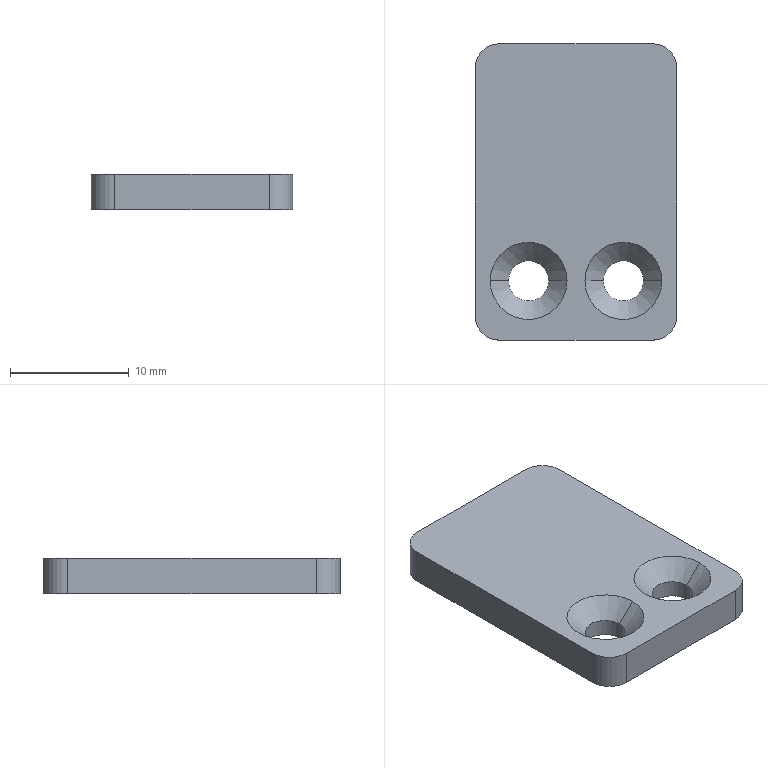Part | NX | features BREP 1 | 1 solid | 18 faces | box 17 x 25 x 3 mm | volume 1177 mm3 | cylinder 8 | plane 6 | cone 4 | commonest cylinder face diameters 3.4 x4 4 x4
STEP:
#1=CARTESIAN_POINT('',(-8.5,10.5,-3.));
#2=VERTEX_POINT('',#1);
#3=CARTESIAN_POINT('',(-6.5,12.5,-3.));
#4=VERTEX_POINT('',#3);
#5=CARTESIAN_POINT('',(-6.5,10.5,-3.));
#6=DIRECTION('',(0.,0.,-1.));
#7=DIRECTION('',(-1.,0.,0.));
#8=AXIS2_PLACEMENT_3D('',#5,#6,#7);
#9=CIRCLE('',#8,2.);
#10=EDGE_CURVE('',#2,#4,#9,.T.);
#11=ORIENTED_EDGE('',*,*,#10,.F.);
#12=CARTESIAN_POINT('',(-8.5,10.5,0.));
#13=VERTEX_POINT('',#12);
#14=CARTESIAN_POINT('',(-8.5,10.5,-3.));
#15=DIRECTION('',(0.,0.,-1.));
#16=VECTOR('',#15,1000.);
#17=LINE('',#14,#16);
#18=EDGE_CURVE('',#13,#2,#17,.T.);
#19=ORIENTED_EDGE('',*,*,#18,.F.);
#20=CARTESIAN_POINT('',(-6.5,12.5,0.));
#21=VERTEX_POINT('',#20);
#22=CARTESIAN_POINT('',(-6.5,10.5,0.));
#23=DIRECTION('',(0.,0.,1.));
#24=DIRECTION('',(-1.,0.,0.));
#25=AXIS2_PLACEMENT_3D('',#22,#23,#24);
#26=CIRCLE('',#25,2.);
#27=EDGE_CURVE('',#21,#13,#26,.T.);
#28=ORIENTED_EDGE('',*,*,#27,.F.);
#29=CARTESIAN_POINT('',(-6.5,12.5,-3.));
#30=DIRECTION('',(0.,0.,1.));
#31=VECTOR('',#30,1000.);
#32=LINE('',#29,#31);
#33=EDGE_CURVE('',#4,#21,#32,.T.);
#34=ORIENTED_EDGE('',*,*,#33,.F.);
#35=EDGE_LOOP('',(#11,#19,#28,#34));
#36=FACE_BOUND('',#35,.T.);
#37=CARTESIAN_POINT('',(-6.5,10.5,-3.));
#38=DIRECTION('',(0.,0.,1.));
#39=DIRECTION('',(1.,0.,0.));
#40=AXIS2_PLACEMENT_3D('',#37,#38,#39);
#41=CYLINDRICAL_SURFACE('',#40,2.);
#42=ADVANCED_FACE('',(#36),#41,.T.);
#43=CARTESIAN_POINT('',(6.5,12.5,-3.));
#44=VERTEX_POINT('',#43);
#45=CARTESIAN_POINT('',(8.5,10.5,-3.));
#46=VERTEX_POINT('',#45);
#47=CARTESIAN_POINT('',(6.5,10.5,-3.));
#48=DIRECTION('',(0.,0.,-1.));
#49=DIRECTION('',(-1.,0.,0.));
#50=AXIS2_PLACEMENT_3D('',#47,#48,#49);
#51=CIRCLE('',#50,2.);
#52=EDGE_CURVE('',#44,#46,#51,.T.);
#53=ORIENTED_EDGE('',*,*,#52,.F.);
#54=CARTESIAN_POINT('',(6.5,12.5,0.));
#55=VERTEX_POINT('',#54);
#56=CARTESIAN_POINT('',(6.5,12.5,-3.));
#57=DIRECTION('',(0.,0.,-1.));
#58=VECTOR('',#57,1000.);
#59=LINE('',#56,#58);
#60=EDGE_CURVE('',#55,#44,#59,.T.);
#61=ORIENTED_EDGE('',*,*,#60,.F.);
#62=CARTESIAN_POINT('',(8.5,10.5,0.));
#63=VERTEX_POINT('',#62);
#64=CARTESIAN_POINT('',(6.5,10.5,0.));
#65=DIRECTION('',(0.,0.,1.));
#66=DIRECTION('',(-1.,0.,0.));
#67=AXIS2_PLACEMENT_3D('',#64,#65,#66);
#68=CIRCLE('',#67,2.);
#69=EDGE_CURVE('',#63,#55,#68,.T.);
#70=ORIENTED_EDGE('',*,*,#69,.F.);
#71=CARTESIAN_POINT('',(8.5,10.5,-3.));
#72=DIRECTION('',(0.,0.,1.));
#73=VECTOR('',#72,1000.);
#74=LINE('',#71,#73);
#75=EDGE_CURVE('',#46,#63,#74,.T.);
#76=ORIENTED_EDGE('',*,*,#75,.F.);
#77=EDGE_LOOP('',(#53,#61,#70,#76));
#78=FACE_BOUND('',#77,.T.);
#79=CARTESIAN_POINT('',(6.5,10.5,-3.));
#80=DIRECTION('',(0.,0.,1.));
#81=DIRECTION('',(1.,0.,0.));
#82=AXIS2_PLACEMENT_3D('',#79,#80,#81);
#83=CYLINDRICAL_SURFACE('',#82,2.);
#84=ADVANCED_FACE('',(#78),#83,.T.);
#85=CARTESIAN_POINT('',(-6.5,-12.5,-3.));
#86=VERTEX_POINT('',#85);
#87=CARTESIAN_POINT('',(-8.5,-10.5,-3.));
#88=VERTEX_POINT('',#87);
#89=CARTESIAN_POINT('',(-6.5,-10.5,-3.));
#90=DIRECTION('',(0.,0.,-1.));
#91=DIRECTION('',(-1.,0.,0.));
#92=AXIS2_PLACEMENT_3D('',#89,#90,#91);
#93=CIRCLE('',#92,2.);
#94=EDGE_CURVE('',#86,#88,#93,.T.);
#95=ORIENTED_EDGE('',*,*,#94,.F.);
#96=CARTESIAN_POINT('',(-6.5,-12.5,0.));
#97=VERTEX_POINT('',#96);
#98=CARTESIAN_POINT('',(-6.5,-12.5,-3.));
#99=DIRECTION('',(0.,0.,-1.));
#100=VECTOR('',#99,1000.);
#101=LINE('',#98,#100);
#102=EDGE_CURVE('',#97,#86,#101,.T.);
#103=ORIENTED_EDGE('',*,*,#102,.F.);
#104=CARTESIAN_POINT('',(-8.5,-10.5,0.));
#105=VERTEX_POINT('',#104);
#106=CARTESIAN_POINT('',(-6.5,-10.5,0.));
#107=DIRECTION('',(0.,0.,1.));
#108=DIRECTION('',(-1.,0.,0.));
#109=AXIS2_PLACEMENT_3D('',#106,#107,#108);
#110=CIRCLE('',#109,2.);
#111=EDGE_CURVE('',#105,#97,#110,.T.);
#112=ORIENTED_EDGE('',*,*,#111,.F.);
#113=CARTESIAN_POINT('',(-8.5,-10.5,-3.));
#114=DIRECTION('',(0.,0.,1.));
#115=VECTOR('',#114,1000.);
#116=LINE('',#113,#115);
#117=EDGE_CURVE('',#88,#105,#116,.T.);
#118=ORIENTED_EDGE('',*,*,#117,.F.);
#119=EDGE_LOOP('',(#95,#103,#112,#118));
#120=FACE_BOUND('',#119,.T.);
#121=CARTESIAN_POINT('',(-6.5,-10.5,-3.));
#122=DIRECTION('',(0.,0.,1.));
#123=DIRECTION('',(1.,0.,0.));
#124=AXIS2_PLACEMENT_3D('',#121,#122,#123);
#125=CYLINDRICAL_SURFACE('',#124,2.);
#126=ADVANCED_FACE('',(#120),#125,.T.);
#127=CARTESIAN_POINT('',(8.5,-10.5,-3.));
#128=VERTEX_POINT('',#127);
#129=CARTESIAN_POINT('',(6.5,-12.5,-3.));
#130=VERTEX_POINT('',#129);
#131=CARTESIAN_POINT('',(6.5,-10.5,-3.));
#132=DIRECTION('',(0.,0.,-1.));
#133=DIRECTION('',(-1.,0.,0.));
#134=AXIS2_PLACEMENT_3D('',#131,#132,#133);
#135=CIRCLE('',#134,2.);
#136=EDGE_CURVE('',#128,#130,#135,.T.);
#137=ORIENTED_EDGE('',*,*,#136,.F.);
#138=CARTESIAN_POINT('',(8.5,-10.5,0.));
#139=VERTEX_POINT('',#138);
#140=CARTESIAN_POINT('',(8.5,-10.5,-3.));
#141=DIRECTION('',(0.,0.,-1.));
#142=VECTOR('',#141,1000.);
#143=LINE('',#140,#142);
#144=EDGE_CURVE('',#139,#128,#143,.T.);
#145=ORIENTED_EDGE('',*,*,#144,.F.);
#146=CARTESIAN_POINT('',(6.5,-12.5,0.));
#147=VERTEX_POINT('',#146);
#148=CARTESIAN_POINT('',(6.5,-10.5,0.));
#149=DIRECTION('',(0.,0.,1.));
#150=DIRECTION('',(-1.,0.,0.));
#151=AXIS2_PLACEMENT_3D('',#148,#149,#150);
#152=CIRCLE('',#151,2.);
#153=EDGE_CURVE('',#147,#139,#152,.T.);
#154=ORIENTED_EDGE('',*,*,#153,.F.);
#155=CARTESIAN_POINT('',(6.5,-12.5,-3.));
#156=DIRECTION('',(0.,0.,1.));
#157=VECTOR('',#156,1000.);
#158=LINE('',#155,#157);
#159=EDGE_CURVE('',#130,#147,#158,.T.);
#160=ORIENTED_EDGE('',*,*,#159,.F.);
#161=EDGE_LOOP('',(#137,#145,#154,#160));
#162=FACE_BOUND('',#161,.T.);
#163=CARTESIAN_POINT('',(6.5,-10.5,-3.));
#164=DIRECTION('',(0.,0.,1.));
#165=DIRECTION('',(1.,0.,0.));
#166=AXIS2_PLACEMENT_3D('',#163,#164,#165);
#167=CYLINDRICAL_SURFACE('',#166,2.);
#168=ADVANCED_FACE('',(#162),#167,.T.);
#169=CARTESIAN_POINT('',(-7.25,-7.5,0.));
#170=VERTEX_POINT('',#169);
#171=CARTESIAN_POINT('',(-5.7,-7.5,-1.55));
#172=VERTEX_POINT('',#171);
#173=CARTESIAN_POINT('',(-7.25,-7.5,0.));
#174=DIRECTION('',(-0.7071,0.,0.7071));
#175=VECTOR('',#174,1000.);
#176=LINE('',#173,#175);
#177=EDGE_CURVE('',#170,#172,#176,.F.);
#178=ORIENTED_EDGE('',*,*,#177,.T.);
#179=CARTESIAN_POINT('',(-2.3,-7.5,-1.55));
#180=VERTEX_POINT('',#179);
#181=CARTESIAN_POINT('',(-4.,-7.5,-1.55));
#182=DIRECTION('',(0.,0.,1.));
#183=DIRECTION('',(1.,0.,0.));
#184=AXIS2_PLACEMENT_3D('',#181,#182,#183);
#185=CIRCLE('',#184,1.7);
#186=EDGE_CURVE('',#180,#172,#185,.T.);
#187=ORIENTED_EDGE('',*,*,#186,.F.);
#188=CARTESIAN_POINT('',(-0.75,-7.5,0.));
#189=VERTEX_POINT('',#188);
#190=CARTESIAN_POINT('',(-0.75,-7.5,0.));
#191=DIRECTION('',(0.7071,0.,0.7071));
#192=VECTOR('',#191,1000.);
#193=LINE('',#190,#192);
#194=EDGE_CURVE('',#189,#180,#193,.F.);
#195=ORIENTED_EDGE('',*,*,#194,.F.);
#196=CARTESIAN_POINT('',(-4.,-7.5,0.));
#197=DIRECTION('',(0.,0.,1.));
#198=DIRECTION('',(1.,0.,0.));
#199=AXIS2_PLACEMENT_3D('',#196,#197,#198);
#200=CIRCLE('',#199,3.25);
#201=EDGE_CURVE('',#189,#170,#200,.T.);
#202=ORIENTED_EDGE('',*,*,#201,.T.);
#203=EDGE_LOOP('',(#178,#187,#195,#202));
#204=FACE_BOUND('',#203,.T.);
#205=CARTESIAN_POINT('',(-4.,-7.5,0.));
#206=DIRECTION('',(0.,0.,1.));
#207=DIRECTION('',(1.,0.,0.));
#208=AXIS2_PLACEMENT_3D('',#205,#206,#207);
#209=CONICAL_SURFACE('',#208,3.25,0.7854);
#210=ADVANCED_FACE('',(#204),#209,.F.);
#211=CARTESIAN_POINT('',(-5.7,-7.5,-3.));
#212=VERTEX_POINT('',#211);
#213=CARTESIAN_POINT('',(-5.7,-7.5,0.));
#214=DIRECTION('',(0.,0.,1.));
#215=VECTOR('',#214,1000.);
#216=LINE('',#213,#215);
#217=EDGE_CURVE('',#172,#212,#216,.F.);
#218=ORIENTED_EDGE('',*,*,#217,.T.);
#219=CARTESIAN_POINT('',(-2.3,-7.5,-3.));
#220=VERTEX_POINT('',#219);
#221=CARTESIAN_POINT('',(-4.,-7.5,-3.));
#222=DIRECTION('',(0.,0.,-1.));
#223=DIRECTION('',(-1.,0.,0.));
#224=AXIS2_PLACEMENT_3D('',#221,#222,#223);
#225=CIRCLE('',#224,1.7);
#226=EDGE_CURVE('',#212,#220,#225,.T.);
#227=ORIENTED_EDGE('',*,*,#226,.T.);
#228=CARTESIAN_POINT('',(-2.3,-7.5,0.));
#229=DIRECTION('',(0.,0.,1.));
#230=VECTOR('',#229,1000.);
#231=LINE('',#228,#230);
#232=EDGE_CURVE('',#180,#220,#231,.F.);
#233=ORIENTED_EDGE('',*,*,#232,.F.);
#234=ORIENTED_EDGE('',*,*,#186,.T.);
#235=EDGE_LOOP('',(#218,#227,#233,#234));
#236=FACE_BOUND('',#235,.T.);
#237=CARTESIAN_POINT('',(-4.,-7.5,0.));
#238=DIRECTION('',(0.,0.,1.));
#239=DIRECTION('',(1.,0.,0.));
#240=AXIS2_PLACEMENT_3D('',#237,#238,#239);
#241=CYLINDRICAL_SURFACE('',#240,1.7);
#242=ADVANCED_FACE('',(#236),#241,.F.);
#243=CARTESIAN_POINT('',(0.75,-7.5,0.));
#244=VERTEX_POINT('',#243);
#245=CARTESIAN_POINT('',(2.3,-7.5,-1.55));
#246=VERTEX_POINT('',#245);
#247=CARTESIAN_POINT('',(0.75,-7.5,0.));
#248=DIRECTION('',(-0.7071,0.,0.7071));
#249=VECTOR('',#248,1000.);
#250=LINE('',#247,#249);
#251=EDGE_CURVE('',#244,#246,#250,.F.);
#252=ORIENTED_EDGE('',*,*,#251,.T.);
#253=CARTESIAN_POINT('',(5.7,-7.5,-1.55));
#254=VERTEX_POINT('',#253);
#255=CARTESIAN_POINT('',(4.,-7.5,-1.55));
#256=DIRECTION('',(0.,0.,1.));
#257=DIRECTION('',(1.,0.,0.));
#258=AXIS2_PLACEMENT_3D('',#255,#256,#257);
#259=CIRCLE('',#258,1.7);
#260=EDGE_CURVE('',#254,#246,#259,.T.);
#261=ORIENTED_EDGE('',*,*,#260,.F.);
#262=CARTESIAN_POINT('',(7.25,-7.5,0.));
#263=VERTEX_POINT('',#262);
#264=CARTESIAN_POINT('',(7.25,-7.5,0.));
#265=DIRECTION('',(0.7071,0.,0.7071));
#266=VECTOR('',#265,1000.);
#267=LINE('',#264,#266);
#268=EDGE_CURVE('',#263,#254,#267,.F.);
#269=ORIENTED_EDGE('',*,*,#268,.F.);
#270=CARTESIAN_POINT('',(4.,-7.5,0.));
#271=DIRECTION('',(0.,0.,1.));
#272=DIRECTION('',(1.,0.,0.));
#273=AXIS2_PLACEMENT_3D('',#270,#271,#272);
#274=CIRCLE('',#273,3.25);
#275=EDGE_CURVE('',#263,#244,#274,.T.);
#276=ORIENTED_EDGE('',*,*,#275,.T.);
#277=EDGE_LOOP('',(#252,#261,#269,#276));
#278=FACE_BOUND('',#277,.T.);
#279=CARTESIAN_POINT('',(4.,-7.5,0.));
#280=DIRECTION('',(0.,0.,1.));
#281=DIRECTION('',(1.,0.,0.));
#282=AXIS2_PLACEMENT_3D('',#279,#280,#281);
#283=CONICAL_SURFACE('',#282,3.25,0.7854);
#284=ADVANCED_FACE('',(#278),#283,.F.);
#285=CARTESIAN_POINT('',(2.3,-7.5,-3.));
#286=VERTEX_POINT('',#285);
#287=CARTESIAN_POINT('',(2.3,-7.5,0.));
#288=DIRECTION('',(0.,0.,1.));
#289=VECTOR('',#288,1000.);
#290=LINE('',#287,#289);
#291=EDGE_CURVE('',#246,#286,#290,.F.);
#292=ORIENTED_EDGE('',*,*,#291,.T.);
#293=CARTESIAN_POINT('',(5.7,-7.5,-3.));
#294=VERTEX_POINT('',#293);
#295=CARTESIAN_POINT('',(4.,-7.5,-3.));
#296=DIRECTION('',(0.,0.,-1.));
#297=DIRECTION('',(-1.,0.,0.));
#298=AXIS2_PLACEMENT_3D('',#295,#296,#297);
#299=CIRCLE('',#298,1.7);
#300=EDGE_CURVE('',#286,#294,#299,.T.);
#301=ORIENTED_EDGE('',*,*,#300,.T.);
#302=CARTESIAN_POINT('',(5.7,-7.5,0.));
#303=DIRECTION('',(0.,0.,1.));
#304=VECTOR('',#303,1000.);
#305=LINE('',#302,#304);
#306=EDGE_CURVE('',#254,#294,#305,.F.);
#307=ORIENTED_EDGE('',*,*,#306,.F.);
#308=ORIENTED_EDGE('',*,*,#260,.T.);
#309=EDGE_LOOP('',(#292,#301,#307,#308));
#310=FACE_BOUND('',#309,.T.);
#311=CARTESIAN_POINT('',(4.,-7.5,0.));
#312=DIRECTION('',(0.,0.,1.));
#313=DIRECTION('',(1.,0.,0.));
#314=AXIS2_PLACEMENT_3D('',#311,#312,#313);
#315=CYLINDRICAL_SURFACE('',#314,1.7);
#316=ADVANCED_FACE('',(#310),#315,.F.);
#317=CARTESIAN_POINT('',(-8.5,-12.5,0.));
#318=DIRECTION('',(1.,0.,0.));
#319=VECTOR('',#318,1000.);
#320=LINE('',#317,#319);
#321=EDGE_CURVE('',#97,#147,#320,.T.);
#322=ORIENTED_EDGE('',*,*,#321,.T.);
#323=ORIENTED_EDGE('',*,*,#153,.T.);
#324=CARTESIAN_POINT('',(8.5,-12.5,0.));
#325=DIRECTION('',(0.,1.,0.));
#326=VECTOR('',#325,1000.);
#327=LINE('',#324,#326);
#328=EDGE_CURVE('',#139,#63,#327,.T.);
#329=ORIENTED_EDGE('',*,*,#328,.T.);
#330=ORIENTED_EDGE('',*,*,#69,.T.);
#331=CARTESIAN_POINT('',(-8.5,12.5,0.));
#332=DIRECTION('',(-1.,0.,0.));
#333=VECTOR('',#332,1000.);
#334=LINE('',#331,#333);
#335=EDGE_CURVE('',#55,#21,#334,.T.);
#336=ORIENTED_EDGE('',*,*,#335,.T.);
#337=ORIENTED_EDGE('',*,*,#27,.T.);
#338=CARTESIAN_POINT('',(-8.5,-12.5,0.));
#339=DIRECTION('',(0.,-1.,0.));
#340=VECTOR('',#339,1000.);
#341=LINE('',#338,#340);
#342=EDGE_CURVE('',#13,#105,#341,.T.);
#343=ORIENTED_EDGE('',*,*,#342,.T.);
#344=ORIENTED_EDGE('',*,*,#111,.T.);
#345=EDGE_LOOP('',(#322,#323,#329,#330,#336,#337,#343,#344));
#346=FACE_BOUND('',#345,.T.);
#347=ORIENTED_EDGE('',*,*,#275,.F.);
#348=CARTESIAN_POINT('',(4.,-7.5,0.));
#349=DIRECTION('',(0.,0.,1.));
#350=DIRECTION('',(1.,0.,0.));
#351=AXIS2_PLACEMENT_3D('',#348,#349,#350);
#352=CIRCLE('',#351,3.25);
#353=EDGE_CURVE('',#244,#263,#352,.T.);
#354=ORIENTED_EDGE('',*,*,#353,.F.);
#355=EDGE_LOOP('',(#347,#354));
#356=FACE_BOUND('',#355,.T.);
#357=ORIENTED_EDGE('',*,*,#201,.F.);
#358=CARTESIAN_POINT('',(-4.,-7.5,0.));
#359=DIRECTION('',(0.,0.,1.));
#360=DIRECTION('',(1.,0.,0.));
#361=AXIS2_PLACEMENT_3D('',#358,#359,#360);
#362=CIRCLE('',#361,3.25);
#363=EDGE_CURVE('',#170,#189,#362,.T.);
#364=ORIENTED_EDGE('',*,*,#363,.F.);
#365=EDGE_LOOP('',(#357,#364));
#366=FACE_BOUND('',#365,.T.);
#367=CARTESIAN_POINT('',(0.,0.,0.));
#368=DIRECTION('',(0.,0.,-1.));
#369=DIRECTION('',(-1.,0.,0.));
#370=AXIS2_PLACEMENT_3D('',#367,#368,#369);
#371=PLANE('',#370);
#372=ADVANCED_FACE('',(#346,#356,#366),#371,.F.);
#373=CARTESIAN_POINT('',(8.5,-12.5,-3.));
#374=DIRECTION('',(0.,1.,0.));
#375=VECTOR('',#374,1000.);
#376=LINE('',#373,#375);
#377=EDGE_CURVE('',#128,#46,#376,.T.);
#378=ORIENTED_EDGE('',*,*,#377,.F.);
#379=ORIENTED_EDGE('',*,*,#136,.T.);
#380=CARTESIAN_POINT('',(-8.5,-12.5,-3.));
#381=DIRECTION('',(1.,0.,0.));
#382=VECTOR('',#381,1000.);
#383=LINE('',#380,#382);
#384=EDGE_CURVE('',#86,#130,#383,.T.);
#385=ORIENTED_EDGE('',*,*,#384,.F.);
#386=ORIENTED_EDGE('',*,*,#94,.T.);
#387=CARTESIAN_POINT('',(-8.5,-12.5,-3.));
#388=DIRECTION('',(0.,-1.,0.));
#389=VECTOR('',#388,1000.);
#390=LINE('',#387,#389);
#391=EDGE_CURVE('',#2,#88,#390,.T.);
#392=ORIENTED_EDGE('',*,*,#391,.F.);
#393=ORIENTED_EDGE('',*,*,#10,.T.);
#394=CARTESIAN_POINT('',(-8.5,12.5,-3.));
#395=DIRECTION('',(-1.,0.,0.));
#396=VECTOR('',#395,1000.);
#397=LINE('',#394,#396);
#398=EDGE_CURVE('',#44,#4,#397,.T.);
#399=ORIENTED_EDGE('',*,*,#398,.F.);
#400=ORIENTED_EDGE('',*,*,#52,.T.);
#401=EDGE_LOOP('',(#378,#379,#385,#386,#392,#393,#399,#400));
#402=FACE_BOUND('',#401,.T.);
#403=CARTESIAN_POINT('',(4.,-7.5,-3.));
#404=DIRECTION('',(0.,0.,-1.));
#405=DIRECTION('',(-1.,0.,0.));
#406=AXIS2_PLACEMENT_3D('',#403,#404,#405);
#407=CIRCLE('',#406,1.7);
#408=EDGE_CURVE('',#294,#286,#407,.T.);
#409=ORIENTED_EDGE('',*,*,#408,.F.);
#410=ORIENTED_EDGE('',*,*,#300,.F.);
#411=EDGE_LOOP('',(#409,#410));
#412=FACE_BOUND('',#411,.T.);
#413=CARTESIAN_POINT('',(-4.,-7.5,-3.));
#414=DIRECTION('',(0.,0.,-1.));
#415=DIRECTION('',(-1.,0.,0.));
#416=AXIS2_PLACEMENT_3D('',#413,#414,#415);
#417=CIRCLE('',#416,1.7);
#418=EDGE_CURVE('',#220,#212,#417,.T.);
#419=ORIENTED_EDGE('',*,*,#418,.F.);
#420=ORIENTED_EDGE('',*,*,#226,.F.);
#421=EDGE_LOOP('',(#419,#420));
#422=FACE_BOUND('',#421,.T.);
#423=CARTESIAN_POINT('',(0.,0.,-3.));
#424=DIRECTION('',(0.,0.,-1.));
#425=DIRECTION('',(-1.,0.,0.));
#426=AXIS2_PLACEMENT_3D('',#423,#424,#425);
#427=PLANE('',#426);
#428=ADVANCED_FACE('',(#402,#412,#422),#427,.T.);
#429=ORIENTED_EDGE('',*,*,#335,.F.);
#430=ORIENTED_EDGE('',*,*,#60,.T.);
#431=ORIENTED_EDGE('',*,*,#398,.T.);
#432=ORIENTED_EDGE('',*,*,#33,.T.);
#433=EDGE_LOOP('',(#429,#430,#431,#432));
#434=FACE_BOUND('',#433,.T.);
#435=CARTESIAN_POINT('',(-8.5,12.5,-3.));
#436=DIRECTION('',(0.,1.,0.));
#437=DIRECTION('',(0.,0.,1.));
#438=AXIS2_PLACEMENT_3D('',#435,#436,#437);
#439=PLANE('',#438);
#440=ADVANCED_FACE('',(#434),#439,.T.);
#441=ORIENTED_EDGE('',*,*,#391,.T.);
#442=ORIENTED_EDGE('',*,*,#117,.T.);
#443=ORIENTED_EDGE('',*,*,#342,.F.);
#444=ORIENTED_EDGE('',*,*,#18,.T.);
#445=EDGE_LOOP('',(#441,#442,#443,#444));
#446=FACE_BOUND('',#445,.T.);
#447=CARTESIAN_POINT('',(-8.5,-12.5,-3.));
#448=DIRECTION('',(-1.,0.,0.));
#449=DIRECTION('',(0.,0.,1.));
#450=AXIS2_PLACEMENT_3D('',#447,#448,#449);
#451=PLANE('',#450);
#452=ADVANCED_FACE('',(#446),#451,.T.);
#453=ORIENTED_EDGE('',*,*,#384,.T.);
#454=ORIENTED_EDGE('',*,*,#159,.T.);
#455=ORIENTED_EDGE('',*,*,#321,.F.);
#456=ORIENTED_EDGE('',*,*,#102,.T.);
#457=EDGE_LOOP('',(#453,#454,#455,#456));
#458=FACE_BOUND('',#457,.T.);
#459=CARTESIAN_POINT('',(-8.5,-12.5,-3.));
#460=DIRECTION('',(0.,-1.,0.));
#461=DIRECTION('',(0.,0.,-1.));
#462=AXIS2_PLACEMENT_3D('',#459,#460,#461);
#463=PLANE('',#462);
#464=ADVANCED_FACE('',(#458),#463,.T.);
#465=ORIENTED_EDGE('',*,*,#328,.F.);
#466=ORIENTED_EDGE('',*,*,#144,.T.);
#467=ORIENTED_EDGE('',*,*,#377,.T.);
#468=ORIENTED_EDGE('',*,*,#75,.T.);
#469=EDGE_LOOP('',(#465,#466,#467,#468));
#470=FACE_BOUND('',#469,.T.);
#471=CARTESIAN_POINT('',(8.5,-12.5,-3.));
#472=DIRECTION('',(1.,0.,0.));
#473=DIRECTION('',(0.,0.,-1.));
#474=AXIS2_PLACEMENT_3D('',#471,#472,#473);
#475=PLANE('',#474);
#476=ADVANCED_FACE('',(#470),#475,.T.);
#477=ORIENTED_EDGE('',*,*,#408,.T.);
#478=ORIENTED_EDGE('',*,*,#291,.F.);
#479=CARTESIAN_POINT('',(4.,-7.5,-1.55));
#480=DIRECTION('',(0.,0.,1.));
#481=DIRECTION('',(1.,0.,0.));
#482=AXIS2_PLACEMENT_3D('',#479,#480,#481);
#483=CIRCLE('',#482,1.7);
#484=EDGE_CURVE('',#246,#254,#483,.T.);
#485=ORIENTED_EDGE('',*,*,#484,.T.);
#486=ORIENTED_EDGE('',*,*,#306,.T.);
#487=EDGE_LOOP('',(#477,#478,#485,#486));
#488=FACE_BOUND('',#487,.T.);
#489=CARTESIAN_POINT('',(4.,-7.5,0.));
#490=DIRECTION('',(0.,0.,1.));
#491=DIRECTION('',(1.,0.,0.));
#492=AXIS2_PLACEMENT_3D('',#489,#490,#491);
#493=CYLINDRICAL_SURFACE('',#492,1.7);
#494=ADVANCED_FACE('',(#488),#493,.F.);
#495=ORIENTED_EDGE('',*,*,#484,.F.);
#496=ORIENTED_EDGE('',*,*,#251,.F.);
#497=ORIENTED_EDGE('',*,*,#353,.T.);
#498=ORIENTED_EDGE('',*,*,#268,.T.);
#499=EDGE_LOOP('',(#495,#496,#497,#498));
#500=FACE_BOUND('',#499,.T.);
#501=CARTESIAN_POINT('',(4.,-7.5,0.));
#502=DIRECTION('',(0.,0.,1.));
#503=DIRECTION('',(1.,0.,0.));
#504=AXIS2_PLACEMENT_3D('',#501,#502,#503);
#505=CONICAL_SURFACE('',#504,3.25,0.7854);
#506=ADVANCED_FACE('',(#500),#505,.F.);
#507=ORIENTED_EDGE('',*,*,#418,.T.);
#508=ORIENTED_EDGE('',*,*,#217,.F.);
#509=CARTESIAN_POINT('',(-4.,-7.5,-1.55));
#510=DIRECTION('',(0.,0.,1.));
#511=DIRECTION('',(1.,0.,0.));
#512=AXIS2_PLACEMENT_3D('',#509,#510,#511);
#513=CIRCLE('',#512,1.7);
#514=EDGE_CURVE('',#172,#180,#513,.T.);
#515=ORIENTED_EDGE('',*,*,#514,.T.);
#516=ORIENTED_EDGE('',*,*,#232,.T.);
#517=EDGE_LOOP('',(#507,#508,#515,#516));
#518=FACE_BOUND('',#517,.T.);
#519=CARTESIAN_POINT('',(-4.,-7.5,0.));
#520=DIRECTION('',(0.,0.,1.));
#521=DIRECTION('',(1.,0.,0.));
#522=AXIS2_PLACEMENT_3D('',#519,#520,#521);
#523=CYLINDRICAL_SURFACE('',#522,1.7);
#524=ADVANCED_FACE('',(#518),#523,.F.);
#525=ORIENTED_EDGE('',*,*,#514,.F.);
#526=ORIENTED_EDGE('',*,*,#177,.F.);
#527=ORIENTED_EDGE('',*,*,#363,.T.);
#528=ORIENTED_EDGE('',*,*,#194,.T.);
#529=EDGE_LOOP('',(#525,#526,#527,#528));
#530=FACE_BOUND('',#529,.T.);
#531=CARTESIAN_POINT('',(-4.,-7.5,0.));
#532=DIRECTION('',(0.,0.,1.));
#533=DIRECTION('',(1.,0.,0.));
#534=AXIS2_PLACEMENT_3D('',#531,#532,#533);
#535=CONICAL_SURFACE('',#534,3.25,0.7854);
#536=ADVANCED_FACE('',(#530),#535,.F.);
#537=CLOSED_SHELL('',(#42,#84,#126,#168,#210,#242,#284,#316,#372,#428,#440,#452,#464,#476,#494,#506,#524,#536));
#538=MANIFOLD_SOLID_BREP('',#537);
#539=(LENGTH_UNIT()NAMED_UNIT(*)SI_UNIT(.MILLI.,.METRE.));
#540=UNCERTAINTY_MEASURE_WITH_UNIT(LENGTH_MEASURE(0.00001),#539,'','');
#541=(NAMED_UNIT(*)PLANE_ANGLE_UNIT()SI_UNIT($,.RADIAN.));
#542=(NAMED_UNIT(*)SI_UNIT($,.STERADIAN.)SOLID_ANGLE_UNIT());
#543=(GEOMETRIC_REPRESENTATION_CONTEXT(3)GLOBAL_UNCERTAINTY_ASSIGNED_CONTEXT((#540))GLOBAL_UNIT_ASSIGNED_CONTEXT((#539,#541,#542))REPRESENTATION_CONTEXT('',''));
#544=ADVANCED_BREP_SHAPE_REPRESENTATION('',(#538),#543);